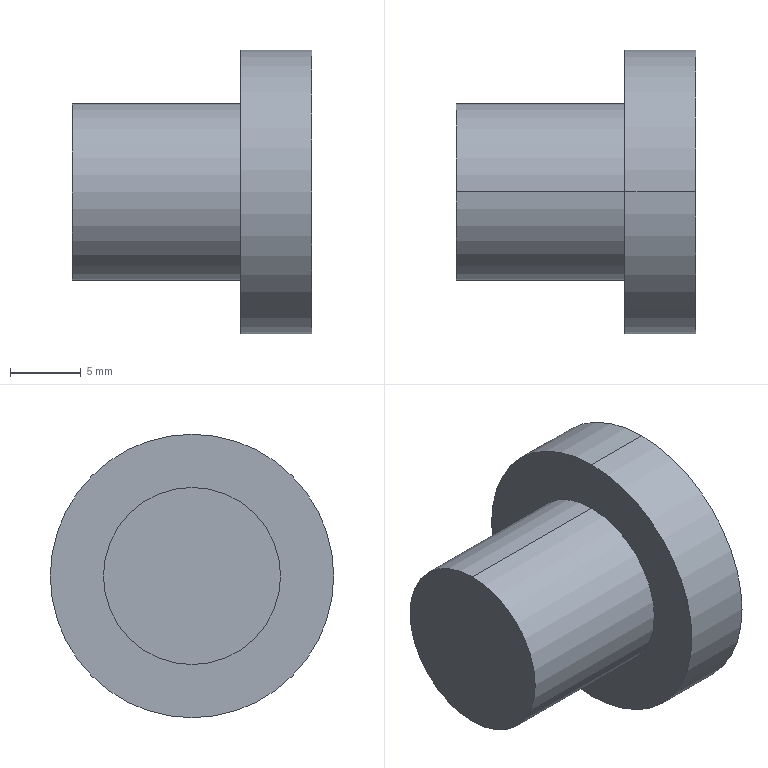Part | SolidWorks | features Revolution 1 | 1 solid | 7 faces | box 16.9 x 20 x 20 mm | volume 3031 mm3 | cylinder 4 | plane 3 | commonest cylinder face diameters 12.5 x2 20 x2
STEP:
#1=CARTESIAN_POINT('',(-568.127,-116.128,10.));
#2=VERTEX_POINT('',#1);
#3=CARTESIAN_POINT('',(-568.127,-116.128,-10.));
#4=VERTEX_POINT('',#3);
#5=CARTESIAN_POINT('',(-568.127,-116.128,0.));
#6=DIRECTION('',(-1.,0.,0.));
#7=DIRECTION('',(0.,0.,1.));
#8=AXIS2_PLACEMENT_3D('',#5,#6,#7);
#9=CIRCLE('',#8,10.);
#10=EDGE_CURVE('',#2,#4,#9,.T.);
#11=ORIENTED_EDGE('',*,*,#10,.T.);
#12=CARTESIAN_POINT('',(-573.127,-116.128,-10.));
#13=VERTEX_POINT('',#12);
#14=CARTESIAN_POINT('',(-585.027,-116.128,-10.));
#15=DIRECTION('',(-1.,0.,0.));
#16=VECTOR('',#15,1000.);
#17=LINE('',#14,#16);
#18=EDGE_CURVE('',#4,#13,#17,.T.);
#19=ORIENTED_EDGE('',*,*,#18,.T.);
#20=CARTESIAN_POINT('',(-573.127,-116.128,10.));
#21=VERTEX_POINT('',#20);
#22=CARTESIAN_POINT('',(-573.127,-116.128,0.));
#23=DIRECTION('',(-1.,0.,0.));
#24=DIRECTION('',(0.,0.,1.));
#25=AXIS2_PLACEMENT_3D('',#22,#23,#24);
#26=CIRCLE('',#25,10.);
#27=EDGE_CURVE('',#21,#13,#26,.T.);
#28=ORIENTED_EDGE('',*,*,#27,.F.);
#29=CARTESIAN_POINT('',(-585.027,-116.128,10.));
#30=DIRECTION('',(-1.,0.,0.));
#31=VECTOR('',#30,1000.);
#32=LINE('',#29,#31);
#33=EDGE_CURVE('',#2,#21,#32,.T.);
#34=ORIENTED_EDGE('',*,*,#33,.F.);
#35=EDGE_LOOP('',(#11,#19,#28,#34));
#36=FACE_OUTER_BOUND('',#35,.T.);
#37=CARTESIAN_POINT('',(-585.027,-116.128,0.));
#38=DIRECTION('',(-1.,0.,0.));
#39=DIRECTION('',(0.,0.,1.));
#40=AXIS2_PLACEMENT_3D('',#37,#38,#39);
#41=CYLINDRICAL_SURFACE('',#40,10.);
#42=ADVANCED_FACE('',(#36),#41,.T.);
#43=CARTESIAN_POINT('',(-573.127,-116.128,6.25));
#44=VERTEX_POINT('',#43);
#45=CARTESIAN_POINT('',(-573.127,-116.128,-6.25));
#46=VERTEX_POINT('',#45);
#47=CARTESIAN_POINT('',(-573.127,-116.128,0.));
#48=DIRECTION('',(-1.,0.,0.));
#49=DIRECTION('',(0.,0.,1.));
#50=AXIS2_PLACEMENT_3D('',#47,#48,#49);
#51=CIRCLE('',#50,6.25);
#52=EDGE_CURVE('',#44,#46,#51,.T.);
#53=ORIENTED_EDGE('',*,*,#52,.T.);
#54=CARTESIAN_POINT('',(-585.027,-116.128,-6.25));
#55=VERTEX_POINT('',#54);
#56=CARTESIAN_POINT('',(-585.027,-116.128,-6.25));
#57=DIRECTION('',(-1.,0.,0.));
#58=VECTOR('',#57,1000.);
#59=LINE('',#56,#58);
#60=EDGE_CURVE('',#46,#55,#59,.T.);
#61=ORIENTED_EDGE('',*,*,#60,.T.);
#62=CARTESIAN_POINT('',(-585.027,-116.128,6.25));
#63=VERTEX_POINT('',#62);
#64=CARTESIAN_POINT('',(-585.027,-116.128,0.));
#65=DIRECTION('',(-1.,0.,0.));
#66=DIRECTION('',(0.,0.,1.));
#67=AXIS2_PLACEMENT_3D('',#64,#65,#66);
#68=CIRCLE('',#67,6.25);
#69=EDGE_CURVE('',#63,#55,#68,.T.);
#70=ORIENTED_EDGE('',*,*,#69,.F.);
#71=CARTESIAN_POINT('',(-585.027,-116.128,6.25));
#72=DIRECTION('',(-1.,0.,0.));
#73=VECTOR('',#72,1000.);
#74=LINE('',#71,#73);
#75=EDGE_CURVE('',#44,#63,#74,.T.);
#76=ORIENTED_EDGE('',*,*,#75,.F.);
#77=EDGE_LOOP('',(#53,#61,#70,#76));
#78=FACE_OUTER_BOUND('',#77,.T.);
#79=CARTESIAN_POINT('',(-585.027,-116.128,0.));
#80=DIRECTION('',(-1.,0.,0.));
#81=DIRECTION('',(0.,0.,1.));
#82=AXIS2_PLACEMENT_3D('',#79,#80,#81);
#83=CYLINDRICAL_SURFACE('',#82,6.25);
#84=ADVANCED_FACE('',(#78),#83,.T.);
#85=ORIENTED_EDGE('',*,*,#69,.T.);
#86=CARTESIAN_POINT('',(-585.027,-116.128,0.));
#87=DIRECTION('',(-1.,0.,0.));
#88=DIRECTION('',(0.,0.,1.));
#89=AXIS2_PLACEMENT_3D('',#86,#87,#88);
#90=CIRCLE('',#89,6.25);
#91=EDGE_CURVE('',#55,#63,#90,.T.);
#92=ORIENTED_EDGE('',*,*,#91,.T.);
#93=EDGE_LOOP('',(#85,#92));
#94=FACE_OUTER_BOUND('',#93,.T.);
#95=CARTESIAN_POINT('',(-585.027,-116.128,0.));
#96=DIRECTION('',(-1.,0.,0.));
#97=DIRECTION('',(0.,0.,1.));
#98=AXIS2_PLACEMENT_3D('',#95,#96,#97);
#99=PLANE('',#98);
#100=ADVANCED_FACE('',(#94),#99,.T.);
#101=ORIENTED_EDGE('',*,*,#60,.F.);
#102=CARTESIAN_POINT('',(-573.127,-116.128,0.));
#103=DIRECTION('',(-1.,0.,0.));
#104=DIRECTION('',(0.,0.,1.));
#105=AXIS2_PLACEMENT_3D('',#102,#103,#104);
#106=CIRCLE('',#105,6.25);
#107=EDGE_CURVE('',#46,#44,#106,.T.);
#108=ORIENTED_EDGE('',*,*,#107,.T.);
#109=ORIENTED_EDGE('',*,*,#75,.T.);
#110=ORIENTED_EDGE('',*,*,#91,.F.);
#111=EDGE_LOOP('',(#101,#108,#109,#110));
#112=FACE_OUTER_BOUND('',#111,.T.);
#113=CARTESIAN_POINT('',(-585.027,-116.128,0.));
#114=DIRECTION('',(-1.,0.,0.));
#115=DIRECTION('',(0.,0.,1.));
#116=AXIS2_PLACEMENT_3D('',#113,#114,#115);
#117=CYLINDRICAL_SURFACE('',#116,6.25);
#118=ADVANCED_FACE('',(#112),#117,.T.);
#119=ORIENTED_EDGE('',*,*,#27,.T.);
#120=CARTESIAN_POINT('',(-573.127,-116.128,0.));
#121=DIRECTION('',(-1.,0.,0.));
#122=DIRECTION('',(0.,0.,1.));
#123=AXIS2_PLACEMENT_3D('',#120,#121,#122);
#124=CIRCLE('',#123,10.);
#125=EDGE_CURVE('',#13,#21,#124,.T.);
#126=ORIENTED_EDGE('',*,*,#125,.T.);
#127=EDGE_LOOP('',(#119,#126));
#128=FACE_OUTER_BOUND('',#127,.T.);
#129=ORIENTED_EDGE('',*,*,#52,.F.);
#130=ORIENTED_EDGE('',*,*,#107,.F.);
#131=EDGE_LOOP('',(#129,#130));
#132=FACE_BOUND('',#131,.T.);
#133=CARTESIAN_POINT('',(-573.127,-122.378,0.));
#134=DIRECTION('',(-1.,0.,0.));
#135=DIRECTION('',(0.,0.,1.));
#136=AXIS2_PLACEMENT_3D('',#133,#134,#135);
#137=PLANE('',#136);
#138=ADVANCED_FACE('',(#128,#132),#137,.T.);
#139=ORIENTED_EDGE('',*,*,#18,.F.);
#140=CARTESIAN_POINT('',(-568.127,-116.128,0.));
#141=DIRECTION('',(-1.,0.,0.));
#142=DIRECTION('',(0.,0.,1.));
#143=AXIS2_PLACEMENT_3D('',#140,#141,#142);
#144=CIRCLE('',#143,10.);
#145=EDGE_CURVE('',#4,#2,#144,.T.);
#146=ORIENTED_EDGE('',*,*,#145,.T.);
#147=ORIENTED_EDGE('',*,*,#33,.T.);
#148=ORIENTED_EDGE('',*,*,#125,.F.);
#149=EDGE_LOOP('',(#139,#146,#147,#148));
#150=FACE_OUTER_BOUND('',#149,.T.);
#151=CARTESIAN_POINT('',(-585.027,-116.128,0.));
#152=DIRECTION('',(-1.,0.,0.));
#153=DIRECTION('',(0.,0.,1.));
#154=AXIS2_PLACEMENT_3D('',#151,#152,#153);
#155=CYLINDRICAL_SURFACE('',#154,10.);
#156=ADVANCED_FACE('',(#150),#155,.T.);
#157=ORIENTED_EDGE('',*,*,#10,.F.);
#158=ORIENTED_EDGE('',*,*,#145,.F.);
#159=EDGE_LOOP('',(#157,#158));
#160=FACE_OUTER_BOUND('',#159,.T.);
#161=CARTESIAN_POINT('',(-568.127,-126.128,0.));
#162=DIRECTION('',(1.,0.,0.));
#163=DIRECTION('',(0.,0.,-1.));
#164=AXIS2_PLACEMENT_3D('',#161,#162,#163);
#165=PLANE('',#164);
#166=ADVANCED_FACE('',(#160),#165,.T.);
#167=CLOSED_SHELL('',(#42,#84,#100,#118,#138,#156,#166));
#168=MANIFOLD_SOLID_BREP('',#167);
#169=CARTESIAN_POINT('',(0.,0.,0.));
#170=DIRECTION('',(0.,0.,1.));
#171=DIRECTION('',(1.,0.,0.));
#172=AXIS2_PLACEMENT_3D('',#169,#170,#171);
#173=(LENGTH_UNIT()NAMED_UNIT(*)SI_UNIT(.MILLI.,.METRE.));
#174=UNCERTAINTY_MEASURE_WITH_UNIT(LENGTH_MEASURE(0.00001),#173,'','');
#175=(NAMED_UNIT(*)PLANE_ANGLE_UNIT()SI_UNIT($,.RADIAN.));
#176=(NAMED_UNIT(*)SI_UNIT($,.STERADIAN.)SOLID_ANGLE_UNIT());
#177=(GEOMETRIC_REPRESENTATION_CONTEXT(3)GLOBAL_UNCERTAINTY_ASSIGNED_CONTEXT((#174))GLOBAL_UNIT_ASSIGNED_CONTEXT((#173,#175,#176))REPRESENTATION_CONTEXT('',''));
#178=ADVANCED_BREP_SHAPE_REPRESENTATION('',(#168,#172),#177);